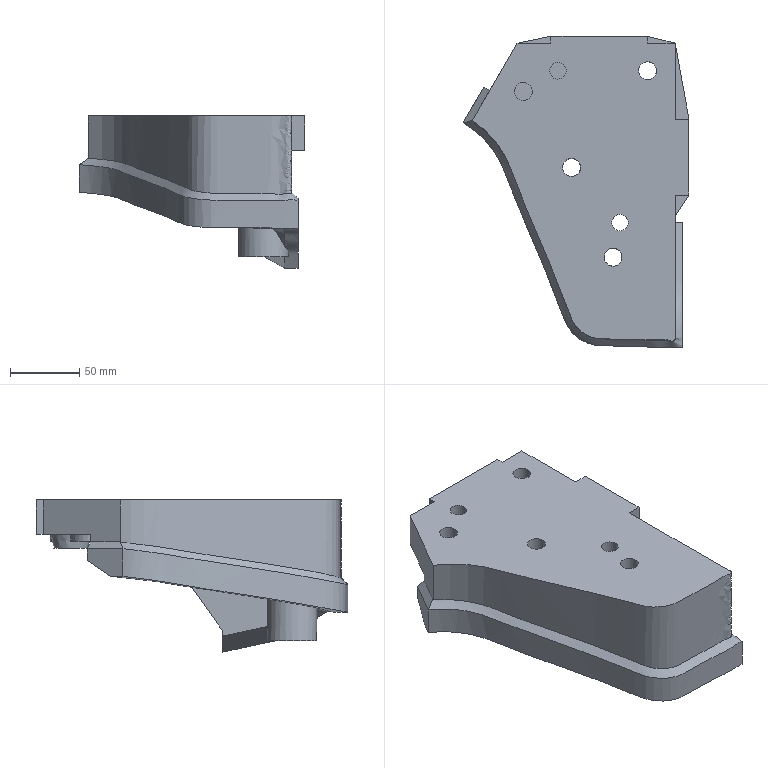Part | NX | features solid 2 | 1 solid | 53 faces | box 163.674 x 225.464 x 110.282 mm | volume 1135622 mm3 | plane 29 | cylinder 14 | spline 8 | cone 2 | commonest cylinder face diameters 13 x6 30 x4 12 x2 16 x1 36 x1